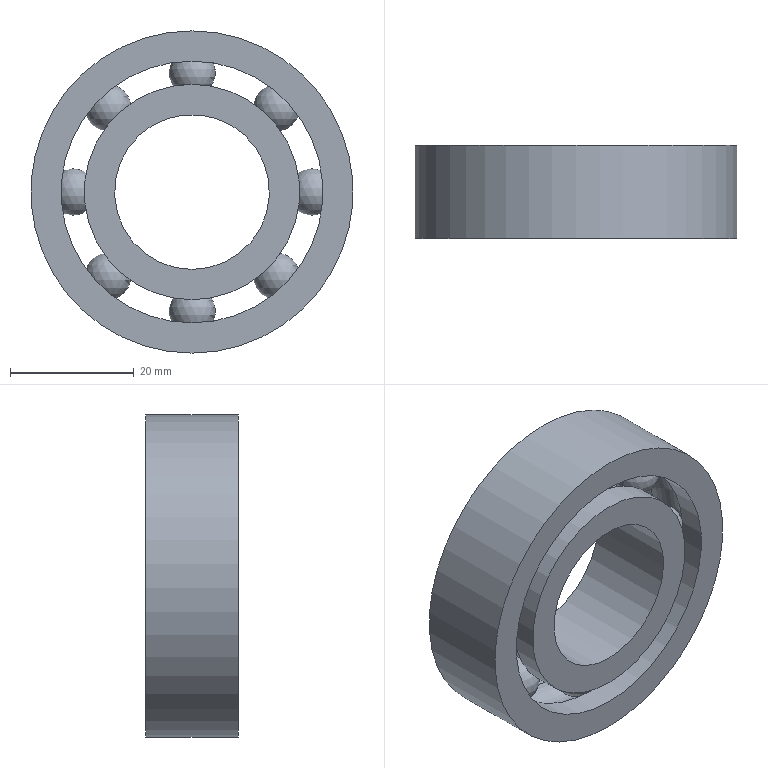Part | NX | features SPHERE 8, Instance Feature 7, DATUM_CSYS 2, Pattern Feature 1, SKETCH 1, SWP104 1 | 10 solids | 20 faces | box 52 x 15 x 52 mm | volume 17377 mm3 | sphere 8 | cylinder 6 | plane 4 | torus 2 | commonest cylinder face diameters 34.76 x2 42.24 x2 25 x1 52 x1
STEP:
#1=CARTESIAN_POINT('',(-13.612,0.,-17.362));
#2=VERTEX_POINT('',#1);
#3=VERTEX_LOOP('',#2);
#4=FACE_BOUND('',#3,.T.);
#5=CARTESIAN_POINT('',(-13.612,0.,-13.612));
#6=DIRECTION('',(0.,0.,1.));
#7=DIRECTION('',(1.,0.,0.));
#8=AXIS2_PLACEMENT_3D('',#5,#6,#7);
#9=SPHERICAL_SURFACE('',#8,3.75);
#10=ADVANCED_FACE('',(#4),#9,.T.);
#11=CLOSED_SHELL('',(#10));
#12=MANIFOLD_SOLID_BREP('',#11);
#13=CARTESIAN_POINT('',(13.612,0.,9.862));
#14=VERTEX_POINT('',#13);
#15=VERTEX_LOOP('',#14);
#16=FACE_BOUND('',#15,.T.);
#17=CARTESIAN_POINT('',(13.612,0.,13.612));
#18=DIRECTION('',(0.,0.,1.));
#19=DIRECTION('',(1.,0.,0.));
#20=AXIS2_PLACEMENT_3D('',#17,#18,#19);
#21=SPHERICAL_SURFACE('',#20,3.75);
#22=ADVANCED_FACE('',(#16),#21,.T.);
#23=CLOSED_SHELL('',(#22));
#24=MANIFOLD_SOLID_BREP('',#23);
#25=CARTESIAN_POINT('',(0.,-7.5,-12.5));
#26=VERTEX_POINT('',#25);
#27=CARTESIAN_POINT('',(0.,-7.5,0.));
#28=DIRECTION('',(0.,-1.,0.));
#29=DIRECTION('',(0.,0.,-1.));
#30=AXIS2_PLACEMENT_3D('',#27,#28,#29);
#31=CIRCLE('',#30,12.5);
#32=EDGE_CURVE('',#26,#26,#31,.T.);
#33=ORIENTED_EDGE('',*,*,#32,.F.);
#34=EDGE_LOOP('',(#33));
#35=FACE_BOUND('',#34,.T.);
#36=CARTESIAN_POINT('',(0.,-7.5,-17.38));
#37=VERTEX_POINT('',#36);
#38=CARTESIAN_POINT('',(0.,-7.5,0.));
#39=DIRECTION('',(0.,-1.,0.));
#40=DIRECTION('',(0.,0.,-1.));
#41=AXIS2_PLACEMENT_3D('',#38,#39,#40);
#42=CIRCLE('',#41,17.38);
#43=EDGE_CURVE('',#37,#37,#42,.T.);
#44=ORIENTED_EDGE('',*,*,#43,.T.);
#45=EDGE_LOOP('',(#44));
#46=FACE_BOUND('',#45,.T.);
#47=CARTESIAN_POINT('',(0.,-7.5,17.38));
#48=DIRECTION('',(0.,1.,0.));
#49=DIRECTION('',(0.,0.,1.));
#50=AXIS2_PLACEMENT_3D('',#47,#48,#49);
#51=PLANE('',#50);
#52=ADVANCED_FACE('',(#35,#46),#51,.F.);
#53=CARTESIAN_POINT('',(0.,7.5,-12.5));
#54=VERTEX_POINT('',#53);
#55=CARTESIAN_POINT('',(0.,7.5,0.));
#56=DIRECTION('',(0.,-1.,0.));
#57=DIRECTION('',(0.,0.,-1.));
#58=AXIS2_PLACEMENT_3D('',#55,#56,#57);
#59=CIRCLE('',#58,12.5);
#60=EDGE_CURVE('',#54,#54,#59,.T.);
#61=ORIENTED_EDGE('',*,*,#60,.F.);
#62=EDGE_LOOP('',(#61));
#63=FACE_BOUND('',#62,.T.);
#64=ORIENTED_EDGE('',*,*,#32,.T.);
#65=EDGE_LOOP('',(#64));
#66=FACE_BOUND('',#65,.T.);
#67=CARTESIAN_POINT('',(0.,0.,0.));
#68=DIRECTION('',(0.,-1.,0.));
#69=DIRECTION('',(0.,0.,-1.));
#70=AXIS2_PLACEMENT_3D('',#67,#68,#69);
#71=CYLINDRICAL_SURFACE('',#70,12.5);
#72=ADVANCED_FACE('',(#63,#66),#71,.F.);
#73=CARTESIAN_POINT('',(0.,7.5,-17.38));
#74=VERTEX_POINT('',#73);
#75=CARTESIAN_POINT('',(0.,7.5,0.));
#76=DIRECTION('',(0.,-1.,0.));
#77=DIRECTION('',(0.,0.,-1.));
#78=AXIS2_PLACEMENT_3D('',#75,#76,#77);
#79=CIRCLE('',#78,17.38);
#80=EDGE_CURVE('',#74,#74,#79,.T.);
#81=ORIENTED_EDGE('',*,*,#80,.F.);
#82=EDGE_LOOP('',(#81));
#83=FACE_BOUND('',#82,.T.);
#84=ORIENTED_EDGE('',*,*,#60,.T.);
#85=EDGE_LOOP('',(#84));
#86=FACE_BOUND('',#85,.T.);
#87=CARTESIAN_POINT('',(0.,7.5,12.5));
#88=DIRECTION('',(0.,-1.,0.));
#89=DIRECTION('',(0.,0.,-1.));
#90=AXIS2_PLACEMENT_3D('',#87,#88,#89);
#91=PLANE('',#90);
#92=ADVANCED_FACE('',(#83,#86),#91,.F.);
#93=CARTESIAN_POINT('',(0.,3.25,-17.38));
#94=VERTEX_POINT('',#93);
#95=CARTESIAN_POINT('',(0.,3.25,0.));
#96=DIRECTION('',(0.,-1.,0.));
#97=DIRECTION('',(0.,0.,-1.));
#98=AXIS2_PLACEMENT_3D('',#95,#96,#97);
#99=CIRCLE('',#98,17.38);
#100=EDGE_CURVE('',#94,#94,#99,.T.);
#101=ORIENTED_EDGE('',*,*,#100,.F.);
#102=EDGE_LOOP('',(#101));
#103=FACE_BOUND('',#102,.T.);
#104=ORIENTED_EDGE('',*,*,#80,.T.);
#105=EDGE_LOOP('',(#104));
#106=FACE_BOUND('',#105,.T.);
#107=CARTESIAN_POINT('',(0.,0.,0.));
#108=DIRECTION('',(0.,-1.,0.));
#109=DIRECTION('',(0.,0.,-1.));
#110=AXIS2_PLACEMENT_3D('',#107,#108,#109);
#111=CYLINDRICAL_SURFACE('',#110,17.38);
#112=ADVANCED_FACE('',(#103,#106),#111,.T.);
#113=CARTESIAN_POINT('',(0.,-3.25,-17.38));
#114=VERTEX_POINT('',#113);
#115=CARTESIAN_POINT('',(0.,-3.25,0.));
#116=DIRECTION('',(0.,-1.,0.));
#117=DIRECTION('',(0.,0.,-1.));
#118=AXIS2_PLACEMENT_3D('',#115,#116,#117);
#119=CIRCLE('',#118,17.38);
#120=EDGE_CURVE('',#114,#114,#119,.T.);
#121=ORIENTED_EDGE('',*,*,#120,.F.);
#122=EDGE_LOOP('',(#121));
#123=FACE_BOUND('',#122,.T.);
#124=ORIENTED_EDGE('',*,*,#100,.T.);
#125=EDGE_LOOP('',(#124));
#126=FACE_BOUND('',#125,.T.);
#127=CARTESIAN_POINT('',(0.,0.,0.));
#128=DIRECTION('',(0.,-1.,0.));
#129=DIRECTION('',(0.,0.,-1.));
#130=AXIS2_PLACEMENT_3D('',#127,#128,#129);
#131=TOROIDAL_SURFACE('',#130,19.25,3.75);
#132=ADVANCED_FACE('',(#123,#126),#131,.F.);
#133=ORIENTED_EDGE('',*,*,#43,.F.);
#134=EDGE_LOOP('',(#133));
#135=FACE_BOUND('',#134,.T.);
#136=ORIENTED_EDGE('',*,*,#120,.T.);
#137=EDGE_LOOP('',(#136));
#138=FACE_BOUND('',#137,.T.);
#139=CARTESIAN_POINT('',(0.,0.,0.));
#140=DIRECTION('',(0.,-1.,0.));
#141=DIRECTION('',(0.,0.,-1.));
#142=AXIS2_PLACEMENT_3D('',#139,#140,#141);
#143=CYLINDRICAL_SURFACE('',#142,17.38);
#144=ADVANCED_FACE('',(#135,#138),#143,.T.);
#145=CLOSED_SHELL('',(#52,#72,#92,#112,#132,#144));
#146=MANIFOLD_SOLID_BREP('',#145);
#147=CARTESIAN_POINT('',(-19.25,0.,-3.75));
#148=VERTEX_POINT('',#147);
#149=VERTEX_LOOP('',#148);
#150=FACE_BOUND('',#149,.T.);
#151=CARTESIAN_POINT('',(-19.25,0.,0.));
#152=DIRECTION('',(0.,0.,1.));
#153=DIRECTION('',(1.,0.,0.));
#154=AXIS2_PLACEMENT_3D('',#151,#152,#153);
#155=SPHERICAL_SURFACE('',#154,3.75);
#156=ADVANCED_FACE('',(#150),#155,.T.);
#157=CLOSED_SHELL('',(#156));
#158=MANIFOLD_SOLID_BREP('',#157);
#159=CARTESIAN_POINT('',(0.,0.,15.5));
#160=VERTEX_POINT('',#159);
#161=VERTEX_LOOP('',#160);
#162=FACE_BOUND('',#161,.T.);
#163=CARTESIAN_POINT('',(0.,0.,19.25));
#164=DIRECTION('',(0.,0.,1.));
#165=DIRECTION('',(1.,0.,0.));
#166=AXIS2_PLACEMENT_3D('',#163,#164,#165);
#167=SPHERICAL_SURFACE('',#166,3.75);
#168=ADVANCED_FACE('',(#162),#167,.T.);
#169=CLOSED_SHELL('',(#168));
#170=MANIFOLD_SOLID_BREP('',#169);
#171=CARTESIAN_POINT('',(13.612,0.,-17.362));
#172=VERTEX_POINT('',#171);
#173=VERTEX_LOOP('',#172);
#174=FACE_BOUND('',#173,.T.);
#175=CARTESIAN_POINT('',(13.612,0.,-13.612));
#176=DIRECTION('',(0.,0.,1.));
#177=DIRECTION('',(1.,0.,0.));
#178=AXIS2_PLACEMENT_3D('',#175,#176,#177);
#179=SPHERICAL_SURFACE('',#178,3.75);
#180=ADVANCED_FACE('',(#174),#179,.T.);
#181=CLOSED_SHELL('',(#180));
#182=MANIFOLD_SOLID_BREP('',#181);
#183=CARTESIAN_POINT('',(0.,-7.5,-21.12));
#184=VERTEX_POINT('',#183);
#185=CARTESIAN_POINT('',(0.,-7.5,0.));
#186=DIRECTION('',(0.,-1.,0.));
#187=DIRECTION('',(0.,0.,-1.));
#188=AXIS2_PLACEMENT_3D('',#185,#186,#187);
#189=CIRCLE('',#188,21.12);
#190=EDGE_CURVE('',#184,#184,#189,.T.);
#191=ORIENTED_EDGE('',*,*,#190,.F.);
#192=EDGE_LOOP('',(#191));
#193=FACE_BOUND('',#192,.T.);
#194=CARTESIAN_POINT('',(0.,-7.5,-26.));
#195=VERTEX_POINT('',#194);
#196=CARTESIAN_POINT('',(0.,-7.5,0.));
#197=DIRECTION('',(0.,-1.,0.));
#198=DIRECTION('',(0.,0.,-1.));
#199=AXIS2_PLACEMENT_3D('',#196,#197,#198);
#200=CIRCLE('',#199,26.);
#201=EDGE_CURVE('',#195,#195,#200,.T.);
#202=ORIENTED_EDGE('',*,*,#201,.T.);
#203=EDGE_LOOP('',(#202));
#204=FACE_BOUND('',#203,.T.);
#205=CARTESIAN_POINT('',(0.,-7.5,26.));
#206=DIRECTION('',(0.,1.,0.));
#207=DIRECTION('',(0.,0.,1.));
#208=AXIS2_PLACEMENT_3D('',#205,#206,#207);
#209=PLANE('',#208);
#210=ADVANCED_FACE('',(#193,#204),#209,.F.);
#211=CARTESIAN_POINT('',(0.,-3.25,-21.12));
#212=VERTEX_POINT('',#211);
#213=CARTESIAN_POINT('',(0.,-3.25,0.));
#214=DIRECTION('',(0.,-1.,0.));
#215=DIRECTION('',(0.,0.,-1.));
#216=AXIS2_PLACEMENT_3D('',#213,#214,#215);
#217=CIRCLE('',#216,21.12);
#218=EDGE_CURVE('',#212,#212,#217,.T.);
#219=ORIENTED_EDGE('',*,*,#218,.F.);
#220=EDGE_LOOP('',(#219));
#221=FACE_BOUND('',#220,.T.);
#222=ORIENTED_EDGE('',*,*,#190,.T.);
#223=EDGE_LOOP('',(#222));
#224=FACE_BOUND('',#223,.T.);
#225=CARTESIAN_POINT('',(0.,0.,0.));
#226=DIRECTION('',(0.,-1.,0.));
#227=DIRECTION('',(0.,0.,-1.));
#228=AXIS2_PLACEMENT_3D('',#225,#226,#227);
#229=CYLINDRICAL_SURFACE('',#228,21.12);
#230=ADVANCED_FACE('',(#221,#224),#229,.F.);
#231=CARTESIAN_POINT('',(0.,3.25,-21.12));
#232=VERTEX_POINT('',#231);
#233=CARTESIAN_POINT('',(0.,3.25,0.));
#234=DIRECTION('',(0.,-1.,0.));
#235=DIRECTION('',(0.,0.,-1.));
#236=AXIS2_PLACEMENT_3D('',#233,#234,#235);
#237=CIRCLE('',#236,21.12);
#238=EDGE_CURVE('',#232,#232,#237,.T.);
#239=ORIENTED_EDGE('',*,*,#238,.F.);
#240=EDGE_LOOP('',(#239));
#241=FACE_BOUND('',#240,.T.);
#242=ORIENTED_EDGE('',*,*,#218,.T.);
#243=EDGE_LOOP('',(#242));
#244=FACE_BOUND('',#243,.T.);
#245=CARTESIAN_POINT('',(0.,0.,0.));
#246=DIRECTION('',(0.,-1.,0.));
#247=DIRECTION('',(0.,0.,-1.));
#248=AXIS2_PLACEMENT_3D('',#245,#246,#247);
#249=TOROIDAL_SURFACE('',#248,19.25,3.75);
#250=ADVANCED_FACE('',(#241,#244),#249,.F.);
#251=CARTESIAN_POINT('',(0.,7.5,-21.12));
#252=VERTEX_POINT('',#251);
#253=CARTESIAN_POINT('',(0.,7.5,0.));
#254=DIRECTION('',(0.,-1.,0.));
#255=DIRECTION('',(0.,0.,-1.));
#256=AXIS2_PLACEMENT_3D('',#253,#254,#255);
#257=CIRCLE('',#256,21.12);
#258=EDGE_CURVE('',#252,#252,#257,.T.);
#259=ORIENTED_EDGE('',*,*,#258,.F.);
#260=EDGE_LOOP('',(#259));
#261=FACE_BOUND('',#260,.T.);
#262=ORIENTED_EDGE('',*,*,#238,.T.);
#263=EDGE_LOOP('',(#262));
#264=FACE_BOUND('',#263,.T.);
#265=CARTESIAN_POINT('',(0.,0.,0.));
#266=DIRECTION('',(0.,-1.,0.));
#267=DIRECTION('',(0.,0.,-1.));
#268=AXIS2_PLACEMENT_3D('',#265,#266,#267);
#269=CYLINDRICAL_SURFACE('',#268,21.12);
#270=ADVANCED_FACE('',(#261,#264),#269,.F.);
#271=CARTESIAN_POINT('',(0.,7.5,-26.));
#272=VERTEX_POINT('',#271);
#273=CARTESIAN_POINT('',(0.,7.5,0.));
#274=DIRECTION('',(0.,-1.,0.));
#275=DIRECTION('',(0.,0.,-1.));
#276=AXIS2_PLACEMENT_3D('',#273,#274,#275);
#277=CIRCLE('',#276,26.);
#278=EDGE_CURVE('',#272,#272,#277,.T.);
#279=ORIENTED_EDGE('',*,*,#278,.F.);
#280=EDGE_LOOP('',(#279));
#281=FACE_BOUND('',#280,.T.);
#282=ORIENTED_EDGE('',*,*,#258,.T.);
#283=EDGE_LOOP('',(#282));
#284=FACE_BOUND('',#283,.T.);
#285=CARTESIAN_POINT('',(0.,7.5,21.12));
#286=DIRECTION('',(0.,-1.,0.));
#287=DIRECTION('',(0.,0.,-1.));
#288=AXIS2_PLACEMENT_3D('',#285,#286,#287);
#289=PLANE('',#288);
#290=ADVANCED_FACE('',(#281,#284),#289,.F.);
#291=ORIENTED_EDGE('',*,*,#201,.F.);
#292=EDGE_LOOP('',(#291));
#293=FACE_BOUND('',#292,.T.);
#294=ORIENTED_EDGE('',*,*,#278,.T.);
#295=EDGE_LOOP('',(#294));
#296=FACE_BOUND('',#295,.T.);
#297=CARTESIAN_POINT('',(0.,0.,0.));
#298=DIRECTION('',(0.,-1.,0.));
#299=DIRECTION('',(0.,0.,-1.));
#300=AXIS2_PLACEMENT_3D('',#297,#298,#299);
#301=CYLINDRICAL_SURFACE('',#300,26.);
#302=ADVANCED_FACE('',(#293,#296),#301,.T.);
#303=CLOSED_SHELL('',(#210,#230,#250,#270,#290,#302));
#304=MANIFOLD_SOLID_BREP('',#303);
#305=CARTESIAN_POINT('',(-13.612,0.,9.862));
#306=VERTEX_POINT('',#305);
#307=VERTEX_LOOP('',#306);
#308=FACE_BOUND('',#307,.T.);
#309=CARTESIAN_POINT('',(-13.612,0.,13.612));
#310=DIRECTION('',(0.,0.,1.));
#311=DIRECTION('',(1.,0.,0.));
#312=AXIS2_PLACEMENT_3D('',#309,#310,#311);
#313=SPHERICAL_SURFACE('',#312,3.75);
#314=ADVANCED_FACE('',(#308),#313,.T.);
#315=CLOSED_SHELL('',(#314));
#316=MANIFOLD_SOLID_BREP('',#315);
#317=CARTESIAN_POINT('',(0.,0.,-23.));
#318=VERTEX_POINT('',#317);
#319=VERTEX_LOOP('',#318);
#320=FACE_BOUND('',#319,.T.);
#321=CARTESIAN_POINT('',(0.,0.,-19.25));
#322=DIRECTION('',(0.,0.,1.));
#323=DIRECTION('',(1.,0.,0.));
#324=AXIS2_PLACEMENT_3D('',#321,#322,#323);
#325=SPHERICAL_SURFACE('',#324,3.75);
#326=ADVANCED_FACE('',(#320),#325,.T.);
#327=CLOSED_SHELL('',(#326));
#328=MANIFOLD_SOLID_BREP('',#327);
#329=CARTESIAN_POINT('',(19.25,0.,-3.75));
#330=VERTEX_POINT('',#329);
#331=VERTEX_LOOP('',#330);
#332=FACE_BOUND('',#331,.T.);
#333=CARTESIAN_POINT('',(19.25,0.,0.));
#334=DIRECTION('',(0.,0.,1.));
#335=DIRECTION('',(1.,0.,0.));
#336=AXIS2_PLACEMENT_3D('',#333,#334,#335);
#337=SPHERICAL_SURFACE('',#336,3.75);
#338=ADVANCED_FACE('',(#332),#337,.T.);
#339=CLOSED_SHELL('',(#338));
#340=MANIFOLD_SOLID_BREP('',#339);
#341=(LENGTH_UNIT()NAMED_UNIT(*)SI_UNIT(.MILLI.,.METRE.));
#342=UNCERTAINTY_MEASURE_WITH_UNIT(LENGTH_MEASURE(0.00001),#341,'','');
#343=(NAMED_UNIT(*)PLANE_ANGLE_UNIT()SI_UNIT($,.RADIAN.));
#344=(NAMED_UNIT(*)SI_UNIT($,.STERADIAN.)SOLID_ANGLE_UNIT());
#345=(GEOMETRIC_REPRESENTATION_CONTEXT(3)GLOBAL_UNCERTAINTY_ASSIGNED_CONTEXT((#342))GLOBAL_UNIT_ASSIGNED_CONTEXT((#341,#343,#344))REPRESENTATION_CONTEXT('',''));
#346=ADVANCED_BREP_SHAPE_REPRESENTATION('',(#12,#24,#146,#158,#170,#182,#304,#316,#328,#340),#345);